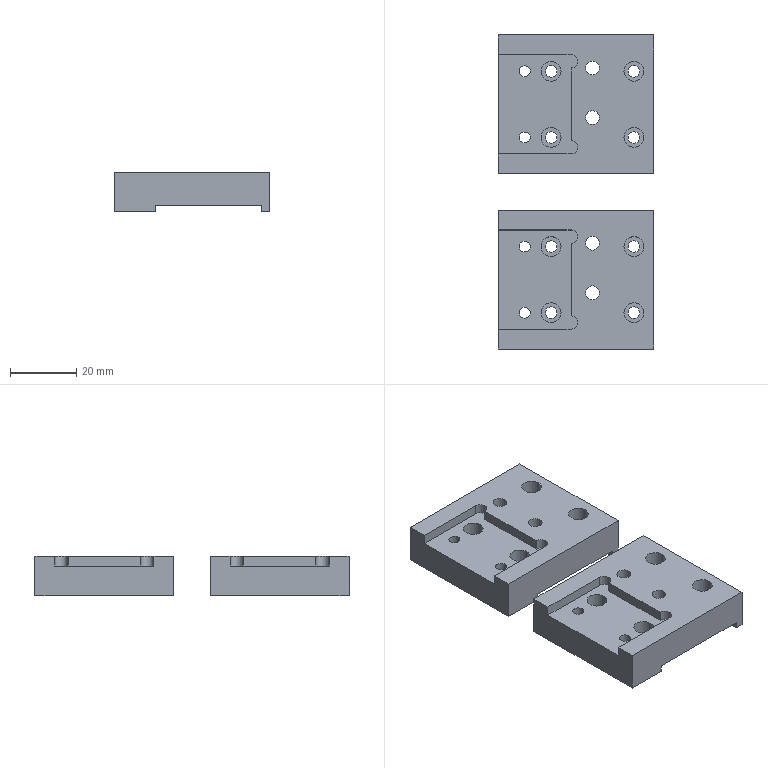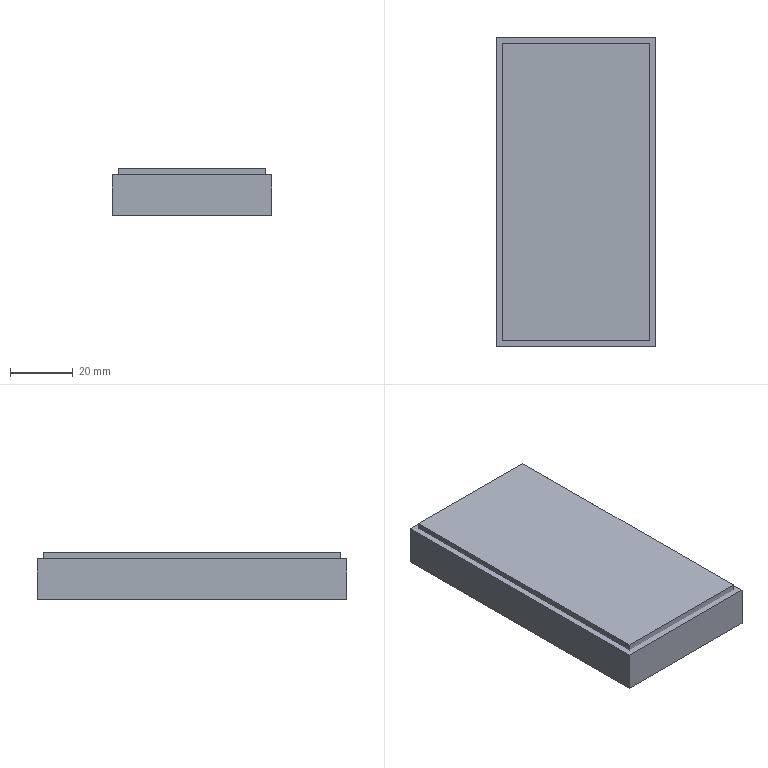CAM job | NX | 3-axis milling, drilling | part box 47 x 95 x 12 mm | stock box 51 x 99 x 15 mm
Tools:
number,name,description,diameter,corner_radius,flute_length,length,flutes
19,D80,Milling Tool-5 Parameters,80.0,0.0,50.0,75.0,2
1,D6A45,Milling Tool-5 Parameters,6.0,0.0,50.0,75.0,2
4,4.2ZT,Drilling Tool,4.2,0.0,35.0,50.0,2
3,3.3ZT,Drilling Tool,3.3,0.0,35.0,50.0,2
7,3.5ZT,Drilling Tool,3.5,0.0,35.0,50.0,2
15,D10,Milling Tool-5 Parameters,10.0,0.0,50.0,75.0,2
14,D10JING,Milling Tool-5 Parameters,10.0,0.0,50.0,75.0,2
11,D4,Milling Tool-5 Parameters,4.0,0.0,30.0,30.0,4
Operations:
program,operation,operation_type,tool,method,geometry_group,spindle_rpm,surface_speed,feed_per_tooth,feed_cut,feed_plunge,cut_length_mm,path_length_mm,cut_time_min,machine_time_min
1,FLOOR_WALL,VolumeBased25DMillingOperation,D80,METHOD,A,6500.0,1633.0,0.1154,1500.0,100.0,191.0,245.0,0.1273,0.1327
1,DRILLING,Operation,D6A45,METHOD,A,5000.0,94.0,0.035,350.0,0.0,64.0,449.08,0.1829,0.2214
1,DRILLING_COPY_COPY,Operation,4.2ZT,METHOD,A,2000.0,26.0,0.075,300.0,0.0,63.047,263.807,0.2102,0.2302
1,DRILLING_COPY,Operation,3.3ZT,METHOD,A,2000.0,20.0,0.05,200.0,0.0,69.966,282.515,0.3498,0.3711
1,DRILLING_COPY_COPY_1,Operation,3.5ZT,METHOD,A,2000.0,20.0,0.05,200.0,0.0,136.412,518.214,0.6821,0.7202
1,ZLEVEL_PROFILE,ZLevelMilling,D10,METHOD,A,9500.0,298.0,0.1579,3000.0,1000.0,5559.456,5826.05,1.917,1.944
1,FLOOR_WALL_1,VolumeBased25DMillingOperation,D10,METHOD,A,9500.0,298.0,0.1579,3000.0,100.0,658.936,896.433,0.2196,0.2434
1,FLOOR_WALL_COPY,VolumeBased25DMillingOperation,D10JING,METHOD,A,9500.0,298.0,0.0789,1500.0,100.0,409.084,572.988,0.2727,0.2891
1,ZLEVEL_PROFILE_COPY_1,ZLevelMilling,D10JING,METHOD,A,9500.0,298.0,0.0632,1200.0,1000.0,937.73,1204.354,0.8674,0.8941
1,HOLE_MILLING,CylinderMilling,D4,METHOD,A,9500.0,119.0,0.0421,1600.0,100.0,956.825,1676.825,0.598,0.67
1,ZLEVEL_PROFILE_COPY,ZLevelMilling,D4,METHOD,A,9500.0,119.0,0.0395,1500.0,1000.0,418.699,841.409,0.3017,0.3439
1,PLANAR_MILL_COPY_COPY_COPY,PlanarMilling,D6A45,METHOD,A,9500.0,179.0,0.0658,1250.0,100.0,598.324,1372.307,0.4787,0.5561
1,刀补,VolumeBased25DMillingOperation,D4,METHOD,A,9500.0,298.0,0.0789,1500.0,100.0,161.859,303.771,0.1079,0.1221
2,FLOOR_WALL_COPY_1,VolumeBased25DMillingOperation,D80,METHOD,B,6500.0,1633.0,0.1154,1500.0,100.0,561.0,1079.001,0.374,0.4258
2,FLOOR_WALL_1_COPY,VolumeBased25DMillingOperation,D10,METHOD,B,9500.0,298.0,0.1579,3000.0,100.0,872.89,1006.991,0.291,0.3044
2,FLOOR_WALL_COPY_COPY,VolumeBased25DMillingOperation,D10JING,METHOD,B,9500.0,298.0,0.0789,1500.0,100.0,923.68,1078.284,0.6158,0.6312
2,PLANAR_MILL_COPY_COPY_COPY_COPY,PlanarMilling,D6A45,METHOD,B,9500.0,179.0,0.0658,1250.0,100.0,474.035,1117.887,0.3792,0.4436
2,刀补_COPY,VolumeBased25DMillingOperation,D4,METHOD,B,9500.0,298.0,0.0789,1500.0,100.0,212.16,384.262,0.1414,0.1587